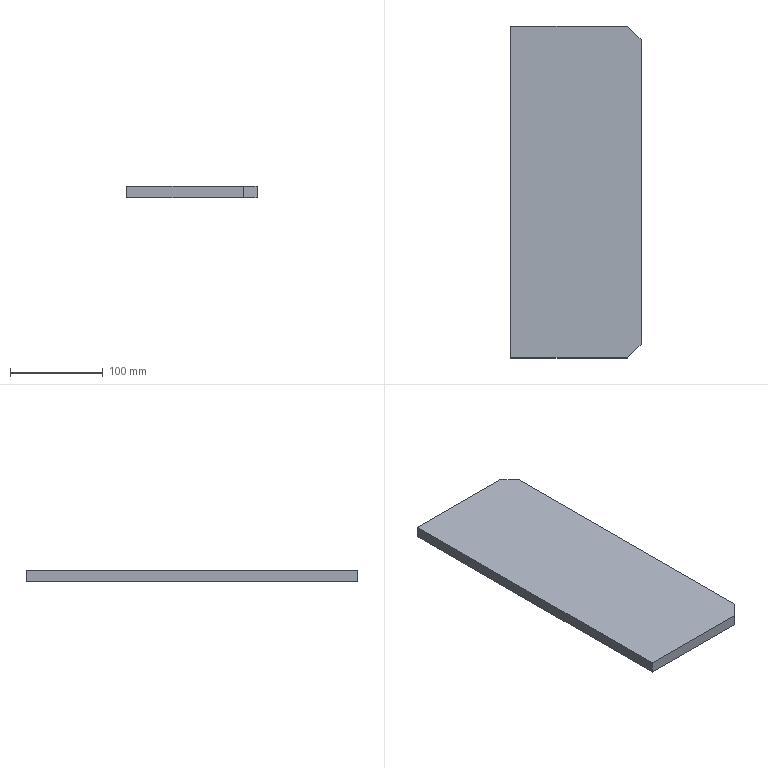Part | SolidWorks | features Chamfer 1, Extrusion 1 | 1 solid | 8 faces | box 140 x 357 x 12 mm | volume 597060 mm3 | plane 8
STEP:
#1=CARTESIAN_POINT('',(0.,357.,0.));
#2=VERTEX_POINT('',#1);
#3=CARTESIAN_POINT('',(0.,0.,0.));
#4=VERTEX_POINT('',#3);
#5=CARTESIAN_POINT('',(0.,0.,0.));
#6=DIRECTION('',(0.,-1.,0.));
#7=VECTOR('',#6,1000.);
#8=LINE('',#5,#7);
#9=EDGE_CURVE('',#2,#4,#8,.T.);
#10=ORIENTED_EDGE('',*,*,#9,.T.);
#11=CARTESIAN_POINT('',(0.,0.,12.));
#12=VERTEX_POINT('',#11);
#13=CARTESIAN_POINT('',(0.,0.,12.));
#14=DIRECTION('',(0.,0.,-1.));
#15=VECTOR('',#14,1000.);
#16=LINE('',#13,#15);
#17=EDGE_CURVE('',#12,#4,#16,.T.);
#18=ORIENTED_EDGE('',*,*,#17,.F.);
#19=CARTESIAN_POINT('',(0.,357.,12.));
#20=VERTEX_POINT('',#19);
#21=CARTESIAN_POINT('',(0.,0.,12.));
#22=DIRECTION('',(0.,-1.,0.));
#23=VECTOR('',#22,1000.);
#24=LINE('',#21,#23);
#25=EDGE_CURVE('',#20,#12,#24,.T.);
#26=ORIENTED_EDGE('',*,*,#25,.F.);
#27=CARTESIAN_POINT('',(0.,357.,12.));
#28=DIRECTION('',(0.,0.,-1.));
#29=VECTOR('',#28,1000.);
#30=LINE('',#27,#29);
#31=EDGE_CURVE('',#20,#2,#30,.T.);
#32=ORIENTED_EDGE('',*,*,#31,.T.);
#33=EDGE_LOOP('',(#10,#18,#26,#32));
#34=FACE_OUTER_BOUND('',#33,.T.);
#35=CARTESIAN_POINT('',(0.,0.,12.));
#36=DIRECTION('',(1.,0.,0.));
#37=DIRECTION('',(0.,0.,-1.));
#38=AXIS2_PLACEMENT_3D('',#35,#36,#37);
#39=PLANE('',#38);
#40=ADVANCED_FACE('',(#34),#39,.F.);
#41=CARTESIAN_POINT('',(125.,0.,0.));
#42=VERTEX_POINT('',#41);
#43=CARTESIAN_POINT('',(0.,0.,0.));
#44=DIRECTION('',(1.,0.,0.));
#45=VECTOR('',#44,1000.);
#46=LINE('',#43,#45);
#47=EDGE_CURVE('',#4,#42,#46,.T.);
#48=ORIENTED_EDGE('',*,*,#47,.T.);
#49=CARTESIAN_POINT('',(125.,0.,12.));
#50=VERTEX_POINT('',#49);
#51=CARTESIAN_POINT('',(125.,0.,12.));
#52=DIRECTION('',(0.,0.,1.));
#53=VECTOR('',#52,1000.);
#54=LINE('',#51,#53);
#55=EDGE_CURVE('',#42,#50,#54,.T.);
#56=ORIENTED_EDGE('',*,*,#55,.T.);
#57=CARTESIAN_POINT('',(0.,0.,12.));
#58=DIRECTION('',(1.,0.,0.));
#59=VECTOR('',#58,1000.);
#60=LINE('',#57,#59);
#61=EDGE_CURVE('',#12,#50,#60,.T.);
#62=ORIENTED_EDGE('',*,*,#61,.F.);
#63=ORIENTED_EDGE('',*,*,#17,.T.);
#64=EDGE_LOOP('',(#48,#56,#62,#63));
#65=FACE_OUTER_BOUND('',#64,.T.);
#66=CARTESIAN_POINT('',(0.,0.,12.));
#67=DIRECTION('',(0.,1.,0.));
#68=DIRECTION('',(0.,0.,1.));
#69=AXIS2_PLACEMENT_3D('',#66,#67,#68);
#70=PLANE('',#69);
#71=ADVANCED_FACE('',(#65),#70,.F.);
#72=CARTESIAN_POINT('',(140.,15.,12.));
#73=VERTEX_POINT('',#72);
#74=CARTESIAN_POINT('',(140.,342.,12.));
#75=VERTEX_POINT('',#74);
#76=CARTESIAN_POINT('',(140.,0.,12.));
#77=DIRECTION('',(0.,1.,0.));
#78=VECTOR('',#77,1000.);
#79=LINE('',#76,#78);
#80=EDGE_CURVE('',#73,#75,#79,.T.);
#81=ORIENTED_EDGE('',*,*,#80,.F.);
#82=CARTESIAN_POINT('',(140.,15.,0.));
#83=VERTEX_POINT('',#82);
#84=CARTESIAN_POINT('',(140.,15.,12.));
#85=DIRECTION('',(0.,0.,-1.));
#86=VECTOR('',#85,1000.);
#87=LINE('',#84,#86);
#88=EDGE_CURVE('',#73,#83,#87,.T.);
#89=ORIENTED_EDGE('',*,*,#88,.T.);
#90=CARTESIAN_POINT('',(140.,342.,0.));
#91=VERTEX_POINT('',#90);
#92=CARTESIAN_POINT('',(140.,0.,0.));
#93=DIRECTION('',(0.,1.,0.));
#94=VECTOR('',#93,1000.);
#95=LINE('',#92,#94);
#96=EDGE_CURVE('',#83,#91,#95,.T.);
#97=ORIENTED_EDGE('',*,*,#96,.T.);
#98=CARTESIAN_POINT('',(140.,342.,12.));
#99=DIRECTION('',(0.,0.,1.));
#100=VECTOR('',#99,1000.);
#101=LINE('',#98,#100);
#102=EDGE_CURVE('',#91,#75,#101,.T.);
#103=ORIENTED_EDGE('',*,*,#102,.T.);
#104=EDGE_LOOP('',(#81,#89,#97,#103));
#105=FACE_OUTER_BOUND('',#104,.T.);
#106=CARTESIAN_POINT('',(140.,0.,12.));
#107=DIRECTION('',(-1.,0.,0.));
#108=DIRECTION('',(0.,0.,1.));
#109=AXIS2_PLACEMENT_3D('',#106,#107,#108);
#110=PLANE('',#109);
#111=ADVANCED_FACE('',(#105),#110,.F.);
#112=CARTESIAN_POINT('',(125.,357.,12.));
#113=VERTEX_POINT('',#112);
#114=CARTESIAN_POINT('',(0.,357.,12.));
#115=DIRECTION('',(-1.,0.,0.));
#116=VECTOR('',#115,1000.);
#117=LINE('',#114,#116);
#118=EDGE_CURVE('',#113,#20,#117,.T.);
#119=ORIENTED_EDGE('',*,*,#118,.F.);
#120=CARTESIAN_POINT('',(125.,357.,0.));
#121=VERTEX_POINT('',#120);
#122=CARTESIAN_POINT('',(125.,357.,12.));
#123=DIRECTION('',(0.,0.,-1.));
#124=VECTOR('',#123,1000.);
#125=LINE('',#122,#124);
#126=EDGE_CURVE('',#113,#121,#125,.T.);
#127=ORIENTED_EDGE('',*,*,#126,.T.);
#128=CARTESIAN_POINT('',(0.,357.,0.));
#129=DIRECTION('',(-1.,0.,0.));
#130=VECTOR('',#129,1000.);
#131=LINE('',#128,#130);
#132=EDGE_CURVE('',#121,#2,#131,.T.);
#133=ORIENTED_EDGE('',*,*,#132,.T.);
#134=ORIENTED_EDGE('',*,*,#31,.F.);
#135=EDGE_LOOP('',(#119,#127,#133,#134));
#136=FACE_OUTER_BOUND('',#135,.T.);
#137=CARTESIAN_POINT('',(0.,357.,12.));
#138=DIRECTION('',(0.,-1.,0.));
#139=DIRECTION('',(0.,0.,-1.));
#140=AXIS2_PLACEMENT_3D('',#137,#138,#139);
#141=PLANE('',#140);
#142=ADVANCED_FACE('',(#136),#141,.F.);
#143=ORIENTED_EDGE('',*,*,#61,.T.);
#144=CARTESIAN_POINT('',(140.,15.,12.));
#145=DIRECTION('',(0.7071,0.7071,0.));
#146=VECTOR('',#145,1000.);
#147=LINE('',#144,#146);
#148=EDGE_CURVE('',#50,#73,#147,.T.);
#149=ORIENTED_EDGE('',*,*,#148,.T.);
#150=ORIENTED_EDGE('',*,*,#80,.T.);
#151=CARTESIAN_POINT('',(125.,357.,12.));
#152=DIRECTION('',(-0.7071,0.7071,0.));
#153=VECTOR('',#152,1000.);
#154=LINE('',#151,#153);
#155=EDGE_CURVE('',#75,#113,#154,.T.);
#156=ORIENTED_EDGE('',*,*,#155,.T.);
#157=ORIENTED_EDGE('',*,*,#118,.T.);
#158=ORIENTED_EDGE('',*,*,#25,.T.);
#159=EDGE_LOOP('',(#143,#149,#150,#156,#157,#158));
#160=FACE_OUTER_BOUND('',#159,.T.);
#161=CARTESIAN_POINT('',(0.,0.,12.));
#162=DIRECTION('',(0.,0.,-1.));
#163=DIRECTION('',(-1.,0.,0.));
#164=AXIS2_PLACEMENT_3D('',#161,#162,#163);
#165=PLANE('',#164);
#166=ADVANCED_FACE('',(#160),#165,.F.);
#167=ORIENTED_EDGE('',*,*,#96,.F.);
#168=CARTESIAN_POINT('',(62.5,-62.5,0.));
#169=DIRECTION('',(-0.7071,-0.7071,0.));
#170=VECTOR('',#169,1000.);
#171=LINE('',#168,#170);
#172=EDGE_CURVE('',#83,#42,#171,.T.);
#173=ORIENTED_EDGE('',*,*,#172,.T.);
#174=ORIENTED_EDGE('',*,*,#47,.F.);
#175=ORIENTED_EDGE('',*,*,#9,.F.);
#176=ORIENTED_EDGE('',*,*,#132,.F.);
#177=CARTESIAN_POINT('',(241.,241.,0.));
#178=DIRECTION('',(0.7071,-0.7071,0.));
#179=VECTOR('',#178,1000.);
#180=LINE('',#177,#179);
#181=EDGE_CURVE('',#121,#91,#180,.T.);
#182=ORIENTED_EDGE('',*,*,#181,.T.);
#183=EDGE_LOOP('',(#167,#173,#174,#175,#176,#182));
#184=FACE_OUTER_BOUND('',#183,.T.);
#185=CARTESIAN_POINT('',(0.,0.,0.));
#186=DIRECTION('',(0.,0.,-1.));
#187=DIRECTION('',(-1.,0.,0.));
#188=AXIS2_PLACEMENT_3D('',#185,#186,#187);
#189=PLANE('',#188);
#190=ADVANCED_FACE('',(#184),#189,.T.);
#191=ORIENTED_EDGE('',*,*,#148,.F.);
#192=ORIENTED_EDGE('',*,*,#55,.F.);
#193=ORIENTED_EDGE('',*,*,#172,.F.);
#194=ORIENTED_EDGE('',*,*,#88,.F.);
#195=EDGE_LOOP('',(#191,#192,#193,#194));
#196=FACE_OUTER_BOUND('',#195,.T.);
#197=CARTESIAN_POINT('',(140.,15.,12.));
#198=DIRECTION('',(-0.7071,0.7071,0.));
#199=DIRECTION('',(0.,0.,-1.));
#200=AXIS2_PLACEMENT_3D('',#197,#198,#199);
#201=PLANE('',#200);
#202=ADVANCED_FACE('',(#196),#201,.F.);
#203=ORIENTED_EDGE('',*,*,#155,.F.);
#204=ORIENTED_EDGE('',*,*,#102,.F.);
#205=ORIENTED_EDGE('',*,*,#181,.F.);
#206=ORIENTED_EDGE('',*,*,#126,.F.);
#207=EDGE_LOOP('',(#203,#204,#205,#206));
#208=FACE_OUTER_BOUND('',#207,.T.);
#209=CARTESIAN_POINT('',(125.,357.,12.));
#210=DIRECTION('',(-0.7071,-0.7071,0.));
#211=DIRECTION('',(0.,0.,-1.));
#212=AXIS2_PLACEMENT_3D('',#209,#210,#211);
#213=PLANE('',#212);
#214=ADVANCED_FACE('',(#208),#213,.F.);
#215=CLOSED_SHELL('',(#40,#71,#111,#142,#166,#190,#202,#214));
#216=MANIFOLD_SOLID_BREP('',#215);
#217=CARTESIAN_POINT('',(0.,0.,0.));
#218=DIRECTION('',(0.,0.,1.));
#219=DIRECTION('',(1.,0.,0.));
#220=AXIS2_PLACEMENT_3D('',#217,#218,#219);
#221=(LENGTH_UNIT()NAMED_UNIT(*)SI_UNIT(.MILLI.,.METRE.));
#222=UNCERTAINTY_MEASURE_WITH_UNIT(LENGTH_MEASURE(0.00001),#221,'','');
#223=(NAMED_UNIT(*)PLANE_ANGLE_UNIT()SI_UNIT($,.RADIAN.));
#224=(NAMED_UNIT(*)SI_UNIT($,.STERADIAN.)SOLID_ANGLE_UNIT());
#225=(GEOMETRIC_REPRESENTATION_CONTEXT(3)GLOBAL_UNCERTAINTY_ASSIGNED_CONTEXT((#222))GLOBAL_UNIT_ASSIGNED_CONTEXT((#221,#223,#224))REPRESENTATION_CONTEXT('',''));
#226=ADVANCED_BREP_SHAPE_REPRESENTATION('',(#216,#220),#225);